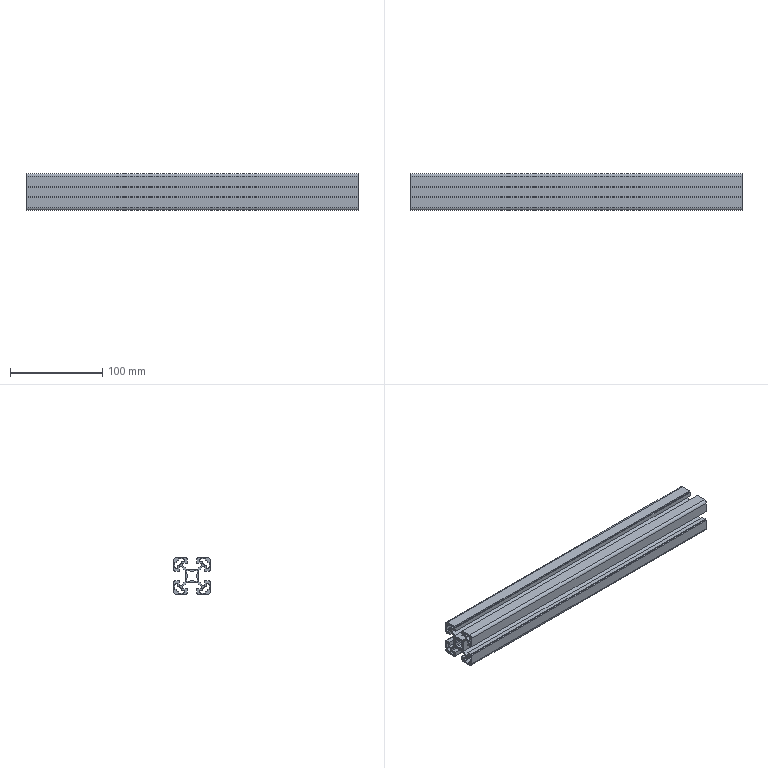Part | STEP file | AL PROFILE 4040 L 360 | 1 solid | 137 faces | box 360 x 40 x 40 mm | volume 200082 mm3 | plane 110 | cylinder 27 | commonest cylinder face diameters 3 x10 5.5 x8 10 x5 6 x4